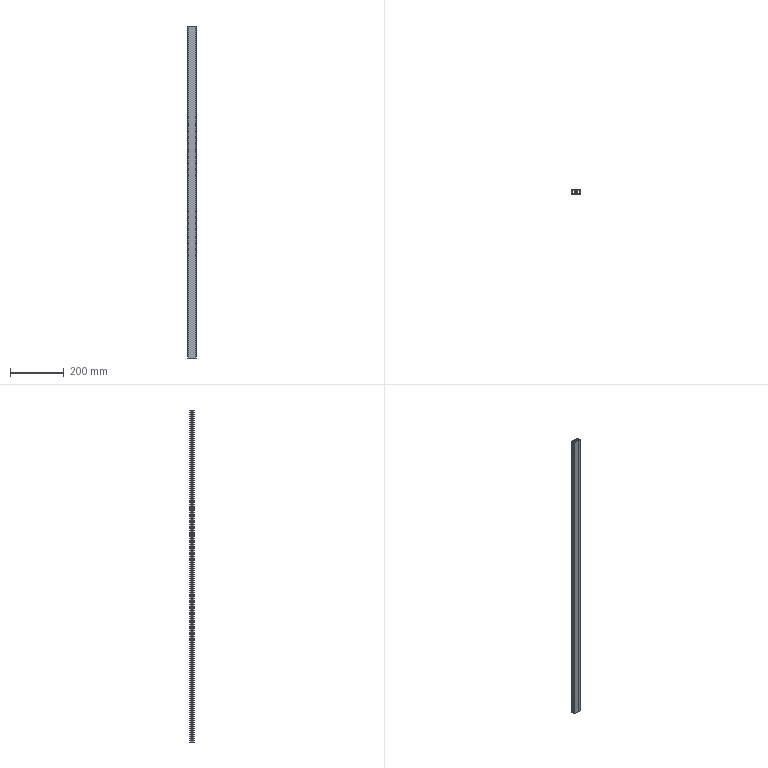Part | SolidWorks | features HoleWzd 3, BaseBody 1, MoveFace 1 | 1 solid | 96 faces | box 30 x 15 x 1236 mm | volume 297813 mm3 | plane 64 | cylinder 32 | commonest cylinder face diameters 1 x12 5 x10 2 x4 6.6 x4 11 x2